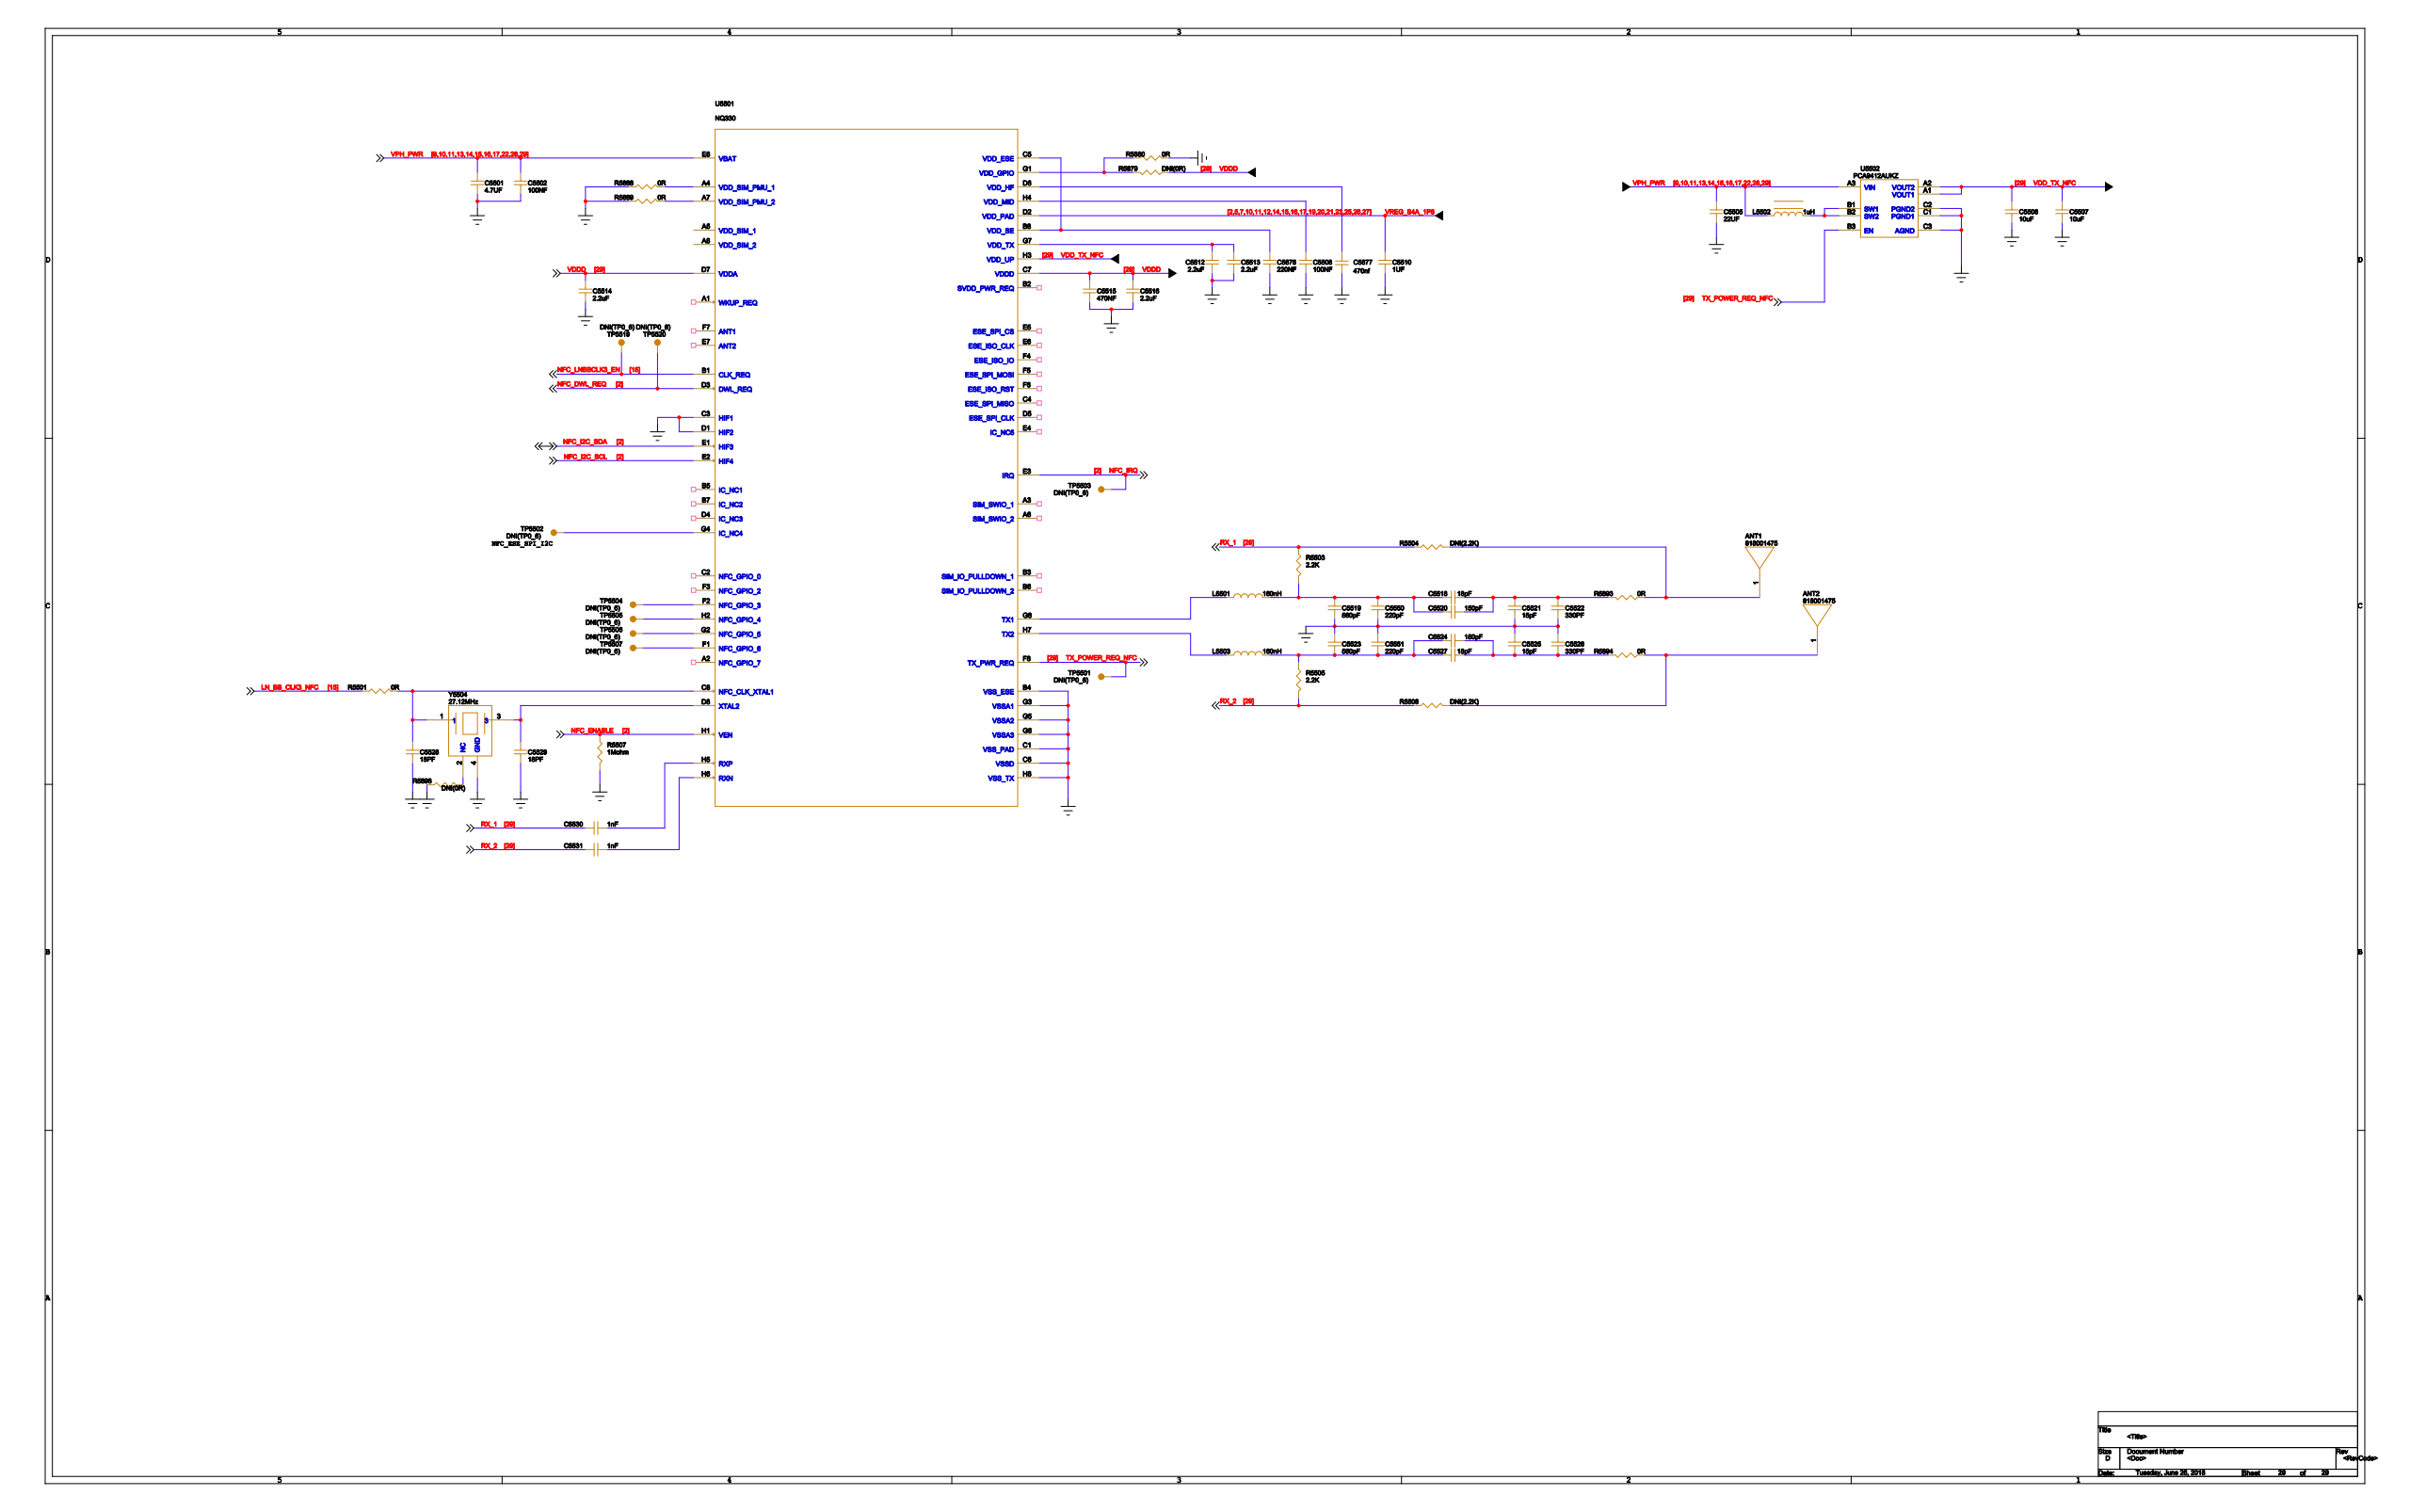Circuit board | Cadence Allegro | 802 parts | 566 nets | one sheet of the schematic
Parts on this sheet (reference | value | footprint):
ANT1 | 818001475 | PIN_ANT_818001475
ANT2 | 818001475 | PIN_ANT_818001475
C5501 | 4.7UF | 0603-BIG
C5502 | 100NF | C0201
C5505 | 22UF | 0603-BIG
C5506 | 10uF | 0603-BIG
C5507 | 10uF | 0603-BIG
C5508 | 100NF | C0201
C5510 | 1UF | C0402
C5512 | 2.2uF | 0402-BIG
C5513 | 2.2uF | 0402-BIG
C5514 | 2.2uF | 0402-BIG
C5515 | 470nF | C0201
C5516 | 2.2uF | 0402-BIG
C5518 | 18pF | C0402
C5519 | 560pF | C0402
C5520 | 150pF | C0201
C5521 | 15pF | C0402
C5522 | 330PF | C0201
C5523 | 560pF | C0402
C5524 | 150pF | C0201
C5525 | 15pF | C0402
C5526 | 330PF | C0201
C5527 | 18pF | C0402
C5528 | 18PF | C0201
C5529 | 18PF | C0201
C5530 | 1nF | C0201
C5531 | 1nF | C0201
C5550 | 220PF | C0201
C5551 | 220PF | C0201
C5876 | 220NF | C0402
C5877 | 470nf | C0402
L5501 | 160nH | L0402_H0P7
L5502 | 1uH | L2016_WPN201610V
L5503 | 160nH | L0402_H0P7
R5501 | 0R | R0201
R5503 | 2.2K | R0201
R5504 | DNI(2.2K) | R0201
R5505 | 2.2K | R0201
R5506 | DNI(2.2K) | R0201
R5507 | 1Mohm | R0201
R5879 | DNI(0R) | R0603
R5880 | 0R | R0201
R5888 | 0R | R0201
R5889 | 0R | R0201
R5893 | 0R | R0603
R5894 | 0R | R0603
R5898 | DNI(0R) | R0201
TP5501 | DNI(TP0_6) | TP_C0P6
TP5502 | DNI(TP0_6) | TP_C0P6
TP5503 | DNI(TP0_6) | TP_C0P6
TP5504 | DNI(TP0_6) | TP_C0P6
TP5505 | DNI(TP0_6) | TP_C0P6
TP5506 | DNI(TP0_6) | TP_C0P6
TP5507 | DNI(TP0_6) | TP_C0P6
TP5519 | DNI(TP0_6) | TP_C0P6
TP5520 | DNI(TP0_6) | TP_C0P6
U5501 | NQ330 | VFBGA64_4X4X1P0_0P4
U5502 | PCA9412AUKZ | WLCSP9_1P24X1P24X0P665_0P4
Y5504 | 27.12MHz | TZ1897B
Nets of these parts (net: part-pin ...):
GND: C5501-2 C5502-2 C5505-2 C5506-2 C5507-2 C5508-2 C5510-2 C5512-2 C5513-2 C5514-2 C5515-2 C5516-2 C5519-2 C5521-2 C5522-2 C5523-1 C5525-1 C5526-1 C5528-2 C5529-2 C5550-2 C5551-1 C5876-2 C5877-1 R5507-2 R5880-2 R5888-1 R5889-1 R5898-1 U5502-C1 U5502-C2 U5502-C3 Y5504-4 U5501-B4 U5501-C1 U5501-C3 U5501-C6 U5501-D1 U5501-G3 U5501-G5 U5501-G6 U5501-H8
N725614: R5898-2 Y5504-2
VDD_TX_NFC: C5506-1 C5507-1 U5502-A1 U5502-A2 U5501-H3
VPH_PWR: C5501-1 C5502-1 C5505-1 L5502-2 U5502-A3 U5501-E8
N502101: C5508-1 U5501-H4
VREG_S4A_1P8: C5510-1 U5501-D2
VDDD: C5514-1 C5515-1 C5516-1 R5879-1 U5501-C7 U5501-D7
LN_BB_CLK3_NFC: R5501-1
N723947: C5528-1 R5501-2 Y5504-1 U5501-C8
N499373: R5879-2 R5880-1 U5501-G1
N505398: R5888-2 U5501-A4
N505400: R5889-2 U5501-A7
N723951: C5529-1 Y5504-3 U5501-D8
N404549: ANT1-1 R5504-2 R5893-1
N404561: ANT2-1 R5506-2 R5894-1
N501932: C5876-1 U5501-B8 U5501-C5
N404391: C5518-1 C5519-1 C5520-1 C5550-1 L5501-2 R5503-2
N404351: C5523-2 C5524-1 C5527-1 C5551-2 L5503-2 R5505-1
N500555: C5512-1 C5513-1 U5501-G7
N502447: C5877-2 U5501-D6
N404379: C5518-2 C5520-2 C5521-1 C5522-1 R5893-2
N404367: C5524-2 C5525-2 C5526-2 C5527-2 R5894-2
RX_1: C5530-1 R5503-1 R5504-1
N503639: C5530-2 U5501-H5
RX_2: C5531-1 R5505-2 R5506-1
N503651: C5531-2 U5501-H6
N498483: L5501-1 U5501-G8
N498490: L5503-1 U5501-H7
N403481: L5502-1 U5502-B1 U5502-B2
NFC_I2C_SDA: U5501-E1
NFC_I2C_SCL: U5501-E2
NFC_ENABLE: R5507-1 U5501-H1
TX_POWER_REQ_NFC: TP5501-1 U5502-B3 U5501-F8
N504183: TP5502-1 U5501-G4
NFC_IRQ: TP5503-1 U5501-E3
N504119: TP5504-1 U5501-F2
N504131: TP5505-1 U5501-H2
N504143: TP5506-1 U5501-G2
N504155: TP5507-1 U5501-F1
NFC_LNBBCLK3_EN: TP5519-1 U5501-B1
NFC_DWL_REQ: TP5520-1 U5501-D3
VDD_SIM_1: U5501-A5
VDD_SIM_2: U5501-A8